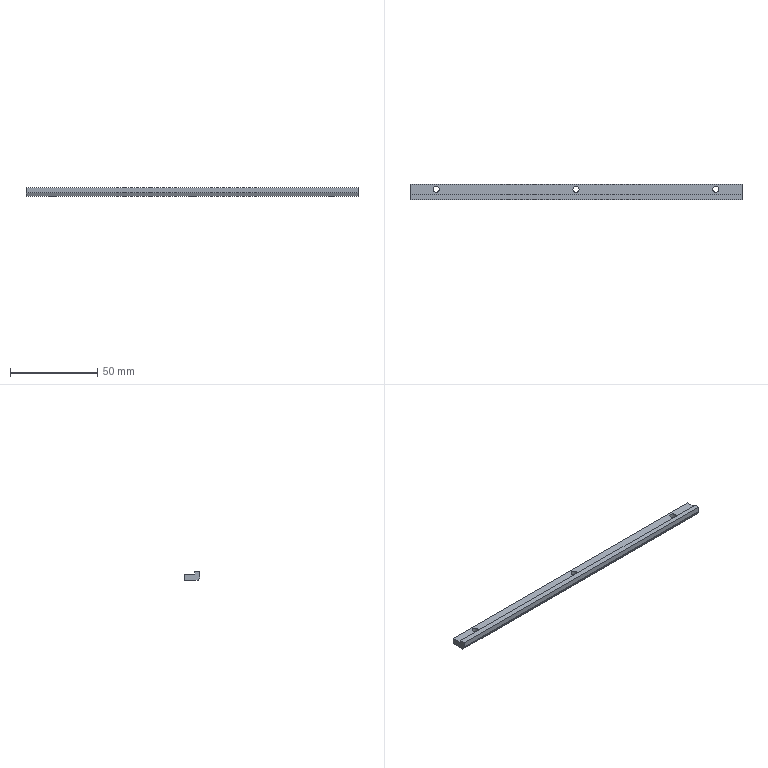Part | SolidWorks | features BaseBody 1 | 1 solid | 15 faces | box 190 x 9 x 5 mm | volume 6549 mm3 | plane 9 | cylinder 6 | commonest cylinder face diameters 3.5 x6
STEP:
#1=CARTESIAN_POINT('',(37.384,150.499,3.5));
#2=VERTEX_POINT('',#1);
#3=CARTESIAN_POINT('',(33.884,150.499,3.5));
#4=VERTEX_POINT('',#3);
#5=CARTESIAN_POINT('',(35.634,150.499,3.5));
#6=DIRECTION('',(0.,0.,-1.));
#7=DIRECTION('',(-1.,0.,0.));
#8=AXIS2_PLACEMENT_3D('',#5,#6,#7);
#9=CIRCLE('',#8,1.75);
#10=EDGE_CURVE('',#2,#4,#9,.T.);
#11=ORIENTED_EDGE('',*,*,#10,.F.);
#12=CARTESIAN_POINT('',(37.384,150.499,0.));
#13=VERTEX_POINT('',#12);
#14=CARTESIAN_POINT('',(37.384,150.499,190.279));
#15=DIRECTION('',(0.,0.,-1.));
#16=VECTOR('',#15,1000.);
#17=LINE('',#14,#16);
#18=EDGE_CURVE('',#2,#13,#17,.T.);
#19=ORIENTED_EDGE('',*,*,#18,.T.);
#20=CARTESIAN_POINT('',(33.884,150.499,0.));
#21=VERTEX_POINT('',#20);
#22=CARTESIAN_POINT('',(35.634,150.499,0.));
#23=DIRECTION('',(0.,0.,-1.));
#24=DIRECTION('',(-1.,0.,0.));
#25=AXIS2_PLACEMENT_3D('',#22,#23,#24);
#26=CIRCLE('',#25,1.75);
#27=EDGE_CURVE('',#13,#21,#26,.T.);
#28=ORIENTED_EDGE('',*,*,#27,.T.);
#29=CARTESIAN_POINT('',(33.884,150.499,190.279));
#30=DIRECTION('',(0.,0.,-1.));
#31=VECTOR('',#30,1000.);
#32=LINE('',#29,#31);
#33=EDGE_CURVE('',#4,#21,#32,.T.);
#34=ORIENTED_EDGE('',*,*,#33,.F.);
#35=EDGE_LOOP('',(#11,#19,#28,#34));
#36=FACE_OUTER_BOUND('',#35,.T.);
#37=CARTESIAN_POINT('',(35.634,150.499,190.279));
#38=DIRECTION('',(0.,0.,-1.));
#39=DIRECTION('',(-1.,0.,0.));
#40=AXIS2_PLACEMENT_3D('',#37,#38,#39);
#41=CYLINDRICAL_SURFACE('',#40,1.75);
#42=ADVANCED_FACE('',(#36),#41,.F.);
#43=CARTESIAN_POINT('',(-122.616,150.499,3.5));
#44=VERTEX_POINT('',#43);
#45=CARTESIAN_POINT('',(-126.116,150.499,3.5));
#46=VERTEX_POINT('',#45);
#47=CARTESIAN_POINT('',(-124.366,150.499,3.5));
#48=DIRECTION('',(0.,0.,-1.));
#49=DIRECTION('',(-1.,0.,0.));
#50=AXIS2_PLACEMENT_3D('',#47,#48,#49);
#51=CIRCLE('',#50,1.75);
#52=EDGE_CURVE('',#44,#46,#51,.T.);
#53=ORIENTED_EDGE('',*,*,#52,.F.);
#54=CARTESIAN_POINT('',(-122.616,150.499,0.));
#55=VERTEX_POINT('',#54);
#56=CARTESIAN_POINT('',(-122.616,150.499,190.279));
#57=DIRECTION('',(0.,0.,-1.));
#58=VECTOR('',#57,1000.);
#59=LINE('',#56,#58);
#60=EDGE_CURVE('',#44,#55,#59,.T.);
#61=ORIENTED_EDGE('',*,*,#60,.T.);
#62=CARTESIAN_POINT('',(-126.116,150.499,0.));
#63=VERTEX_POINT('',#62);
#64=CARTESIAN_POINT('',(-124.366,150.499,0.));
#65=DIRECTION('',(0.,0.,-1.));
#66=DIRECTION('',(-1.,0.,0.));
#67=AXIS2_PLACEMENT_3D('',#64,#65,#66);
#68=CIRCLE('',#67,1.75);
#69=EDGE_CURVE('',#55,#63,#68,.T.);
#70=ORIENTED_EDGE('',*,*,#69,.T.);
#71=CARTESIAN_POINT('',(-126.116,150.499,190.279));
#72=DIRECTION('',(0.,0.,-1.));
#73=VECTOR('',#72,1000.);
#74=LINE('',#71,#73);
#75=EDGE_CURVE('',#46,#63,#74,.T.);
#76=ORIENTED_EDGE('',*,*,#75,.F.);
#77=EDGE_LOOP('',(#53,#61,#70,#76));
#78=FACE_OUTER_BOUND('',#77,.T.);
#79=CARTESIAN_POINT('',(-124.366,150.499,190.279));
#80=DIRECTION('',(0.,0.,-1.));
#81=DIRECTION('',(-1.,0.,0.));
#82=AXIS2_PLACEMENT_3D('',#79,#80,#81);
#83=CYLINDRICAL_SURFACE('',#82,1.75);
#84=ADVANCED_FACE('',(#78),#83,.F.);
#85=CARTESIAN_POINT('',(-42.616,150.499,3.5));
#86=VERTEX_POINT('',#85);
#87=CARTESIAN_POINT('',(-46.116,150.499,3.5));
#88=VERTEX_POINT('',#87);
#89=CARTESIAN_POINT('',(-44.366,150.499,3.5));
#90=DIRECTION('',(0.,0.,-1.));
#91=DIRECTION('',(-1.,0.,0.));
#92=AXIS2_PLACEMENT_3D('',#89,#90,#91);
#93=CIRCLE('',#92,1.75);
#94=EDGE_CURVE('',#86,#88,#93,.T.);
#95=ORIENTED_EDGE('',*,*,#94,.F.);
#96=CARTESIAN_POINT('',(-42.616,150.499,0.));
#97=VERTEX_POINT('',#96);
#98=CARTESIAN_POINT('',(-42.616,150.499,190.279));
#99=DIRECTION('',(0.,0.,-1.));
#100=VECTOR('',#99,1000.);
#101=LINE('',#98,#100);
#102=EDGE_CURVE('',#86,#97,#101,.T.);
#103=ORIENTED_EDGE('',*,*,#102,.T.);
#104=CARTESIAN_POINT('',(-46.116,150.499,0.));
#105=VERTEX_POINT('',#104);
#106=CARTESIAN_POINT('',(-44.366,150.499,0.));
#107=DIRECTION('',(0.,0.,-1.));
#108=DIRECTION('',(-1.,0.,0.));
#109=AXIS2_PLACEMENT_3D('',#106,#107,#108);
#110=CIRCLE('',#109,1.75);
#111=EDGE_CURVE('',#97,#105,#110,.T.);
#112=ORIENTED_EDGE('',*,*,#111,.T.);
#113=CARTESIAN_POINT('',(-46.116,150.499,190.279));
#114=DIRECTION('',(0.,0.,-1.));
#115=VECTOR('',#114,1000.);
#116=LINE('',#113,#115);
#117=EDGE_CURVE('',#88,#105,#116,.T.);
#118=ORIENTED_EDGE('',*,*,#117,.F.);
#119=EDGE_LOOP('',(#95,#103,#112,#118));
#120=FACE_OUTER_BOUND('',#119,.T.);
#121=CARTESIAN_POINT('',(-44.366,150.499,190.279));
#122=DIRECTION('',(0.,0.,-1.));
#123=DIRECTION('',(-1.,0.,0.));
#124=AXIS2_PLACEMENT_3D('',#121,#122,#123);
#125=CYLINDRICAL_SURFACE('',#124,1.75);
#126=ADVANCED_FACE('',(#120),#125,.F.);
#127=CARTESIAN_POINT('',(35.634,150.499,0.));
#128=DIRECTION('',(0.,0.,-1.));
#129=DIRECTION('',(-1.,0.,0.));
#130=AXIS2_PLACEMENT_3D('',#127,#128,#129);
#131=CIRCLE('',#130,1.75);
#132=EDGE_CURVE('',#21,#13,#131,.T.);
#133=ORIENTED_EDGE('',*,*,#132,.F.);
#134=ORIENTED_EDGE('',*,*,#27,.F.);
#135=EDGE_LOOP('',(#133,#134));
#136=FACE_BOUND('',#135,.T.);
#137=CARTESIAN_POINT('',(-124.366,150.499,0.));
#138=DIRECTION('',(0.,0.,-1.));
#139=DIRECTION('',(-1.,0.,0.));
#140=AXIS2_PLACEMENT_3D('',#137,#138,#139);
#141=CIRCLE('',#140,1.75);
#142=EDGE_CURVE('',#63,#55,#141,.T.);
#143=ORIENTED_EDGE('',*,*,#142,.F.);
#144=ORIENTED_EDGE('',*,*,#69,.F.);
#145=EDGE_LOOP('',(#143,#144));
#146=FACE_BOUND('',#145,.T.);
#147=CARTESIAN_POINT('',(-44.366,150.499,0.));
#148=DIRECTION('',(0.,0.,-1.));
#149=DIRECTION('',(-1.,0.,0.));
#150=AXIS2_PLACEMENT_3D('',#147,#148,#149);
#151=CIRCLE('',#150,1.75);
#152=EDGE_CURVE('',#105,#97,#151,.T.);
#153=ORIENTED_EDGE('',*,*,#152,.F.);
#154=ORIENTED_EDGE('',*,*,#111,.F.);
#155=EDGE_LOOP('',(#153,#154));
#156=FACE_BOUND('',#155,.T.);
#157=CARTESIAN_POINT('',(-139.366,153.499,0.));
#158=VERTEX_POINT('',#157);
#159=CARTESIAN_POINT('',(-139.366,145.499,0.));
#160=VERTEX_POINT('',#159);
#161=CARTESIAN_POINT('',(-139.366,148.999,0.));
#162=DIRECTION('',(0.,-1.,0.));
#163=VECTOR('',#162,1000.);
#164=LINE('',#161,#163);
#165=EDGE_CURVE('',#158,#160,#164,.T.);
#166=ORIENTED_EDGE('',*,*,#165,.F.);
#167=CARTESIAN_POINT('',(50.634,153.499,0.));
#168=VERTEX_POINT('',#167);
#169=CARTESIAN_POINT('',(-44.366,153.499,0.));
#170=DIRECTION('',(-1.,0.,0.));
#171=VECTOR('',#170,1000.);
#172=LINE('',#169,#171);
#173=EDGE_CURVE('',#168,#158,#172,.T.);
#174=ORIENTED_EDGE('',*,*,#173,.F.);
#175=CARTESIAN_POINT('',(50.634,145.499,0.));
#176=VERTEX_POINT('',#175);
#177=CARTESIAN_POINT('',(50.634,148.999,0.));
#178=DIRECTION('',(0.,1.,0.));
#179=VECTOR('',#178,1000.);
#180=LINE('',#177,#179);
#181=EDGE_CURVE('',#176,#168,#180,.T.);
#182=ORIENTED_EDGE('',*,*,#181,.F.);
#183=CARTESIAN_POINT('',(-44.366,145.499,0.));
#184=DIRECTION('',(1.,0.,0.));
#185=VECTOR('',#184,1000.);
#186=LINE('',#183,#185);
#187=EDGE_CURVE('',#160,#176,#186,.T.);
#188=ORIENTED_EDGE('',*,*,#187,.F.);
#189=EDGE_LOOP('',(#166,#174,#182,#188));
#190=FACE_OUTER_BOUND('',#189,.T.);
#191=CARTESIAN_POINT('',(-44.366,148.999,0.));
#192=DIRECTION('',(0.,0.,1.));
#193=DIRECTION('',(1.,0.,0.));
#194=AXIS2_PLACEMENT_3D('',#191,#192,#193);
#195=PLANE('',#194);
#196=ADVANCED_FACE('',(#136,#146,#156,#190),#195,.F.);
#197=ORIENTED_EDGE('',*,*,#18,.F.);
#198=CARTESIAN_POINT('',(35.634,150.499,3.5));
#199=DIRECTION('',(0.,0.,-1.));
#200=DIRECTION('',(-1.,0.,0.));
#201=AXIS2_PLACEMENT_3D('',#198,#199,#200);
#202=CIRCLE('',#201,1.75);
#203=EDGE_CURVE('',#4,#2,#202,.T.);
#204=ORIENTED_EDGE('',*,*,#203,.F.);
#205=ORIENTED_EDGE('',*,*,#33,.T.);
#206=ORIENTED_EDGE('',*,*,#132,.T.);
#207=EDGE_LOOP('',(#197,#204,#205,#206));
#208=FACE_OUTER_BOUND('',#207,.T.);
#209=CARTESIAN_POINT('',(35.634,150.499,190.279));
#210=DIRECTION('',(0.,0.,-1.));
#211=DIRECTION('',(-1.,0.,0.));
#212=AXIS2_PLACEMENT_3D('',#209,#210,#211);
#213=CYLINDRICAL_SURFACE('',#212,1.75);
#214=ADVANCED_FACE('',(#208),#213,.F.);
#215=ORIENTED_EDGE('',*,*,#60,.F.);
#216=CARTESIAN_POINT('',(-124.366,150.499,3.5));
#217=DIRECTION('',(0.,0.,-1.));
#218=DIRECTION('',(-1.,0.,0.));
#219=AXIS2_PLACEMENT_3D('',#216,#217,#218);
#220=CIRCLE('',#219,1.75);
#221=EDGE_CURVE('',#46,#44,#220,.T.);
#222=ORIENTED_EDGE('',*,*,#221,.F.);
#223=ORIENTED_EDGE('',*,*,#75,.T.);
#224=ORIENTED_EDGE('',*,*,#142,.T.);
#225=EDGE_LOOP('',(#215,#222,#223,#224));
#226=FACE_OUTER_BOUND('',#225,.T.);
#227=CARTESIAN_POINT('',(-124.366,150.499,190.279));
#228=DIRECTION('',(0.,0.,-1.));
#229=DIRECTION('',(-1.,0.,0.));
#230=AXIS2_PLACEMENT_3D('',#227,#228,#229);
#231=CYLINDRICAL_SURFACE('',#230,1.75);
#232=ADVANCED_FACE('',(#226),#231,.F.);
#233=ORIENTED_EDGE('',*,*,#102,.F.);
#234=CARTESIAN_POINT('',(-44.366,150.499,3.5));
#235=DIRECTION('',(0.,0.,-1.));
#236=DIRECTION('',(-1.,0.,0.));
#237=AXIS2_PLACEMENT_3D('',#234,#235,#236);
#238=CIRCLE('',#237,1.75);
#239=EDGE_CURVE('',#88,#86,#238,.T.);
#240=ORIENTED_EDGE('',*,*,#239,.F.);
#241=ORIENTED_EDGE('',*,*,#117,.T.);
#242=ORIENTED_EDGE('',*,*,#152,.T.);
#243=EDGE_LOOP('',(#233,#240,#241,#242));
#244=FACE_OUTER_BOUND('',#243,.T.);
#245=CARTESIAN_POINT('',(-44.366,150.499,190.279));
#246=DIRECTION('',(0.,0.,-1.));
#247=DIRECTION('',(-1.,0.,0.));
#248=AXIS2_PLACEMENT_3D('',#245,#246,#247);
#249=CYLINDRICAL_SURFACE('',#248,1.75);
#250=ADVANCED_FACE('',(#244),#249,.F.);
#251=CARTESIAN_POINT('',(50.634,144.499,2.));
#252=VERTEX_POINT('',#251);
#253=CARTESIAN_POINT('',(50.634,144.999,1.));
#254=DIRECTION('',(0.,-0.4472,0.8944));
#255=VECTOR('',#254,1000.);
#256=LINE('',#253,#255);
#257=EDGE_CURVE('',#176,#252,#256,.T.);
#258=ORIENTED_EDGE('',*,*,#257,.T.);
#259=CARTESIAN_POINT('',(-139.366,144.499,2.));
#260=VERTEX_POINT('',#259);
#261=CARTESIAN_POINT('',(3.134,144.499,2.));
#262=DIRECTION('',(-1.,0.,0.));
#263=VECTOR('',#262,1000.);
#264=LINE('',#261,#263);
#265=EDGE_CURVE('',#252,#260,#264,.T.);
#266=ORIENTED_EDGE('',*,*,#265,.T.);
#267=CARTESIAN_POINT('',(-139.366,144.999,1.));
#268=DIRECTION('',(0.,0.4472,-0.8944));
#269=VECTOR('',#268,1000.);
#270=LINE('',#267,#269);
#271=EDGE_CURVE('',#260,#160,#270,.T.);
#272=ORIENTED_EDGE('',*,*,#271,.T.);
#273=ORIENTED_EDGE('',*,*,#187,.T.);
#274=EDGE_LOOP('',(#258,#266,#272,#273));
#275=FACE_OUTER_BOUND('',#274,.T.);
#276=CARTESIAN_POINT('',(3.134,144.999,1.));
#277=DIRECTION('',(0.,-0.8944,-0.4472));
#278=DIRECTION('',(0.,0.4472,-0.8944));
#279=AXIS2_PLACEMENT_3D('',#276,#277,#278);
#280=PLANE('',#279);
#281=ADVANCED_FACE('',(#275),#280,.T.);
#282=CARTESIAN_POINT('',(-139.366,153.499,3.5));
#283=VERTEX_POINT('',#282);
#284=CARTESIAN_POINT('',(-139.366,153.499,0.));
#285=DIRECTION('',(0.,0.,-1.));
#286=VECTOR('',#285,1000.);
#287=LINE('',#284,#286);
#288=EDGE_CURVE('',#283,#158,#287,.T.);
#289=ORIENTED_EDGE('',*,*,#288,.T.);
#290=ORIENTED_EDGE('',*,*,#165,.T.);
#291=ORIENTED_EDGE('',*,*,#271,.F.);
#292=CARTESIAN_POINT('',(-139.366,144.499,5.));
#293=VERTEX_POINT('',#292);
#294=CARTESIAN_POINT('',(-139.366,144.499,0.));
#295=DIRECTION('',(0.,0.,1.));
#296=VECTOR('',#295,1000.);
#297=LINE('',#294,#296);
#298=EDGE_CURVE('',#260,#293,#297,.T.);
#299=ORIENTED_EDGE('',*,*,#298,.T.);
#300=CARTESIAN_POINT('',(-139.366,147.499,5.));
#301=VERTEX_POINT('',#300);
#302=CARTESIAN_POINT('',(-139.366,144.499,5.));
#303=DIRECTION('',(0.,1.,0.));
#304=VECTOR('',#303,1000.);
#305=LINE('',#302,#304);
#306=EDGE_CURVE('',#293,#301,#305,.T.);
#307=ORIENTED_EDGE('',*,*,#306,.T.);
#308=CARTESIAN_POINT('',(-139.366,147.499,3.5));
#309=VERTEX_POINT('',#308);
#310=CARTESIAN_POINT('',(-139.366,147.499,5.));
#311=DIRECTION('',(0.,0.,-1.));
#312=VECTOR('',#311,1000.);
#313=LINE('',#310,#312);
#314=EDGE_CURVE('',#301,#309,#313,.T.);
#315=ORIENTED_EDGE('',*,*,#314,.T.);
#316=CARTESIAN_POINT('',(-139.366,144.499,3.5));
#317=DIRECTION('',(0.,1.,0.));
#318=VECTOR('',#317,1000.);
#319=LINE('',#316,#318);
#320=EDGE_CURVE('',#309,#283,#319,.T.);
#321=ORIENTED_EDGE('',*,*,#320,.T.);
#322=EDGE_LOOP('',(#289,#290,#291,#299,#307,#315,#321));
#323=FACE_OUTER_BOUND('',#322,.T.);
#324=CARTESIAN_POINT('',(-139.366,144.499,0.));
#325=DIRECTION('',(-1.,0.,0.));
#326=DIRECTION('',(0.,0.,1.));
#327=AXIS2_PLACEMENT_3D('',#324,#325,#326);
#328=PLANE('',#327);
#329=ADVANCED_FACE('',(#323),#328,.T.);
#330=ORIENTED_EDGE('',*,*,#173,.T.);
#331=ORIENTED_EDGE('',*,*,#288,.F.);
#332=CARTESIAN_POINT('',(50.634,153.499,3.5));
#333=VERTEX_POINT('',#332);
#334=CARTESIAN_POINT('',(-139.366,153.499,3.5));
#335=DIRECTION('',(1.,0.,0.));
#336=VECTOR('',#335,1000.);
#337=LINE('',#334,#336);
#338=EDGE_CURVE('',#283,#333,#337,.T.);
#339=ORIENTED_EDGE('',*,*,#338,.T.);
#340=CARTESIAN_POINT('',(50.634,153.499,0.));
#341=DIRECTION('',(0.,0.,-1.));
#342=VECTOR('',#341,1000.);
#343=LINE('',#340,#342);
#344=EDGE_CURVE('',#333,#168,#343,.T.);
#345=ORIENTED_EDGE('',*,*,#344,.T.);
#346=EDGE_LOOP('',(#330,#331,#339,#345));
#347=FACE_OUTER_BOUND('',#346,.T.);
#348=CARTESIAN_POINT('',(-139.366,153.499,0.));
#349=DIRECTION('',(0.,1.,0.));
#350=DIRECTION('',(0.,0.,1.));
#351=AXIS2_PLACEMENT_3D('',#348,#349,#350);
#352=PLANE('',#351);
#353=ADVANCED_FACE('',(#347),#352,.T.);
#354=CARTESIAN_POINT('',(50.634,147.499,5.));
#355=VERTEX_POINT('',#354);
#356=CARTESIAN_POINT('',(50.634,144.499,5.));
#357=VERTEX_POINT('',#356);
#358=CARTESIAN_POINT('',(50.634,153.499,5.));
#359=DIRECTION('',(0.,-1.,0.));
#360=VECTOR('',#359,1000.);
#361=LINE('',#358,#360);
#362=EDGE_CURVE('',#355,#357,#361,.T.);
#363=ORIENTED_EDGE('',*,*,#362,.T.);
#364=CARTESIAN_POINT('',(50.634,144.499,0.));
#365=DIRECTION('',(0.,0.,-1.));
#366=VECTOR('',#365,1000.);
#367=LINE('',#364,#366);
#368=EDGE_CURVE('',#357,#252,#367,.T.);
#369=ORIENTED_EDGE('',*,*,#368,.T.);
#370=ORIENTED_EDGE('',*,*,#257,.F.);
#371=ORIENTED_EDGE('',*,*,#181,.T.);
#372=ORIENTED_EDGE('',*,*,#344,.F.);
#373=CARTESIAN_POINT('',(50.634,147.499,3.5));
#374=VERTEX_POINT('',#373);
#375=CARTESIAN_POINT('',(50.634,153.499,3.5));
#376=DIRECTION('',(0.,-1.,0.));
#377=VECTOR('',#376,1000.);
#378=LINE('',#375,#377);
#379=EDGE_CURVE('',#333,#374,#378,.T.);
#380=ORIENTED_EDGE('',*,*,#379,.T.);
#381=CARTESIAN_POINT('',(50.634,147.499,5.));
#382=DIRECTION('',(0.,0.,1.));
#383=VECTOR('',#382,1000.);
#384=LINE('',#381,#383);
#385=EDGE_CURVE('',#374,#355,#384,.T.);
#386=ORIENTED_EDGE('',*,*,#385,.T.);
#387=EDGE_LOOP('',(#363,#369,#370,#371,#372,#380,#386));
#388=FACE_OUTER_BOUND('',#387,.T.);
#389=CARTESIAN_POINT('',(50.634,153.499,0.));
#390=DIRECTION('',(1.,0.,0.));
#391=DIRECTION('',(0.,0.,-1.));
#392=AXIS2_PLACEMENT_3D('',#389,#390,#391);
#393=PLANE('',#392);
#394=ADVANCED_FACE('',(#388),#393,.T.);
#395=ORIENTED_EDGE('',*,*,#203,.T.);
#396=ORIENTED_EDGE('',*,*,#10,.T.);
#397=EDGE_LOOP('',(#395,#396));
#398=FACE_BOUND('',#397,.T.);
#399=ORIENTED_EDGE('',*,*,#221,.T.);
#400=ORIENTED_EDGE('',*,*,#52,.T.);
#401=EDGE_LOOP('',(#399,#400));
#402=FACE_BOUND('',#401,.T.);
#403=ORIENTED_EDGE('',*,*,#239,.T.);
#404=ORIENTED_EDGE('',*,*,#94,.T.);
#405=EDGE_LOOP('',(#403,#404));
#406=FACE_BOUND('',#405,.T.);
#407=ORIENTED_EDGE('',*,*,#320,.F.);
#408=CARTESIAN_POINT('',(-39.366,147.499,3.5));
#409=DIRECTION('',(1.,0.,0.));
#410=VECTOR('',#409,1000.);
#411=LINE('',#408,#410);
#412=EDGE_CURVE('',#309,#374,#411,.T.);
#413=ORIENTED_EDGE('',*,*,#412,.T.);
#414=ORIENTED_EDGE('',*,*,#379,.F.);
#415=ORIENTED_EDGE('',*,*,#338,.F.);
#416=EDGE_LOOP('',(#407,#413,#414,#415));
#417=FACE_OUTER_BOUND('',#416,.T.);
#418=CARTESIAN_POINT('',(-39.366,150.499,3.5));
#419=DIRECTION('',(0.,0.,1.));
#420=DIRECTION('',(1.,0.,0.));
#421=AXIS2_PLACEMENT_3D('',#418,#419,#420);
#422=PLANE('',#421);
#423=ADVANCED_FACE('',(#398,#402,#406,#417),#422,.T.);
#424=CARTESIAN_POINT('',(50.634,144.499,5.));
#425=DIRECTION('',(-1.,0.,0.));
#426=VECTOR('',#425,1000.);
#427=LINE('',#424,#426);
#428=EDGE_CURVE('',#357,#293,#427,.T.);
#429=ORIENTED_EDGE('',*,*,#428,.T.);
#430=ORIENTED_EDGE('',*,*,#298,.F.);
#431=ORIENTED_EDGE('',*,*,#265,.F.);
#432=ORIENTED_EDGE('',*,*,#368,.F.);
#433=EDGE_LOOP('',(#429,#430,#431,#432));
#434=FACE_OUTER_BOUND('',#433,.T.);
#435=CARTESIAN_POINT('',(50.634,144.499,0.));
#436=DIRECTION('',(0.,-1.,0.));
#437=DIRECTION('',(0.,0.,-1.));
#438=AXIS2_PLACEMENT_3D('',#435,#436,#437);
#439=PLANE('',#438);
#440=ADVANCED_FACE('',(#434),#439,.T.);
#441=ORIENTED_EDGE('',*,*,#428,.F.);
#442=ORIENTED_EDGE('',*,*,#362,.F.);
#443=CARTESIAN_POINT('',(-44.366,147.499,5.));
#444=DIRECTION('',(-1.,0.,0.));
#445=VECTOR('',#444,1000.);
#446=LINE('',#443,#445);
#447=EDGE_CURVE('',#355,#301,#446,.T.);
#448=ORIENTED_EDGE('',*,*,#447,.T.);
#449=ORIENTED_EDGE('',*,*,#306,.F.);
#450=EDGE_LOOP('',(#441,#442,#448,#449));
#451=FACE_OUTER_BOUND('',#450,.T.);
#452=CARTESIAN_POINT('',(-44.366,148.999,5.));
#453=DIRECTION('',(0.,0.,1.));
#454=DIRECTION('',(1.,0.,0.));
#455=AXIS2_PLACEMENT_3D('',#452,#453,#454);
#456=PLANE('',#455);
#457=ADVANCED_FACE('',(#451),#456,.T.);
#458=ORIENTED_EDGE('',*,*,#412,.F.);
#459=ORIENTED_EDGE('',*,*,#314,.F.);
#460=ORIENTED_EDGE('',*,*,#447,.F.);
#461=ORIENTED_EDGE('',*,*,#385,.F.);
#462=EDGE_LOOP('',(#458,#459,#460,#461));
#463=FACE_OUTER_BOUND('',#462,.T.);
#464=CARTESIAN_POINT('',(-139.366,147.499,5.));
#465=DIRECTION('',(0.,-1.,0.));
#466=DIRECTION('',(0.,0.,-1.));
#467=AXIS2_PLACEMENT_3D('',#464,#465,#466);
#468=PLANE('',#467);
#469=ADVANCED_FACE('',(#463),#468,.F.);
#470=CLOSED_SHELL('',(#42,#84,#126,#196,#214,#232,#250,#281,#329,#353,#394,#423,#440,#457,#469));
#471=MANIFOLD_SOLID_BREP('',#470);
#472=CARTESIAN_POINT('',(0.,0.,0.));
#473=DIRECTION('',(0.,0.,1.));
#474=DIRECTION('',(1.,0.,0.));
#475=AXIS2_PLACEMENT_3D('',#472,#473,#474);
#476=(LENGTH_UNIT()NAMED_UNIT(*)SI_UNIT(.MILLI.,.METRE.));
#477=UNCERTAINTY_MEASURE_WITH_UNIT(LENGTH_MEASURE(0.00001),#476,'','');
#478=(NAMED_UNIT(*)PLANE_ANGLE_UNIT()SI_UNIT($,.RADIAN.));
#479=(NAMED_UNIT(*)SI_UNIT($,.STERADIAN.)SOLID_ANGLE_UNIT());
#480=(GEOMETRIC_REPRESENTATION_CONTEXT(3)GLOBAL_UNCERTAINTY_ASSIGNED_CONTEXT((#477))GLOBAL_UNIT_ASSIGNED_CONTEXT((#476,#478,#479))REPRESENTATION_CONTEXT('',''));
#481=ADVANCED_BREP_SHAPE_REPRESENTATION('',(#471,#475),#480);